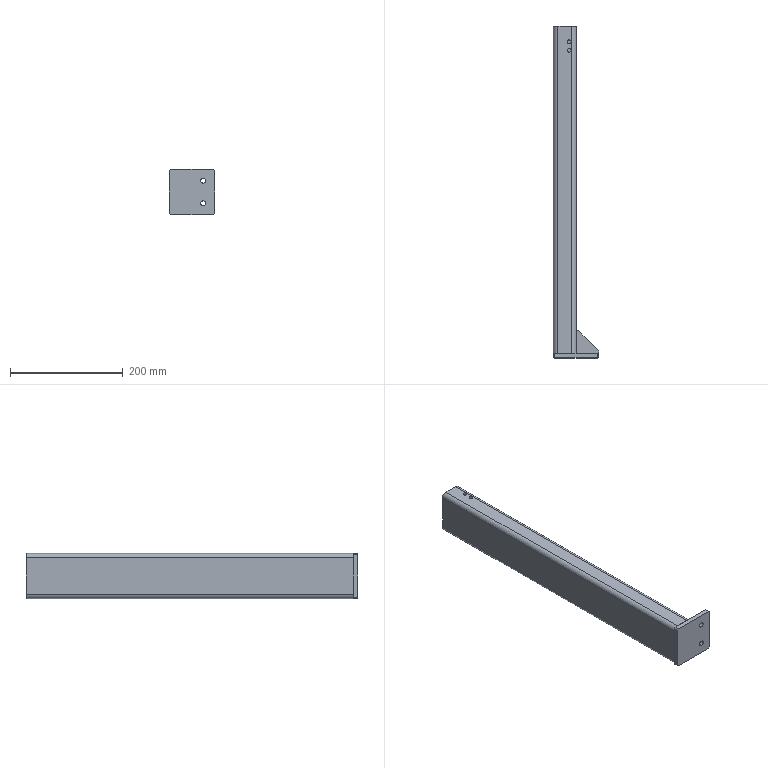Part | SolidWorks | features BaseBody 4 | 4 solids | 57 faces | box 80 x 588 x 80 mm | volume 561871 mm3 | plane 33 | cylinder 24 | commonest cylinder face diameters 5 x4 6 x4 6.8 x4 8 x4 9 x4 16 x4